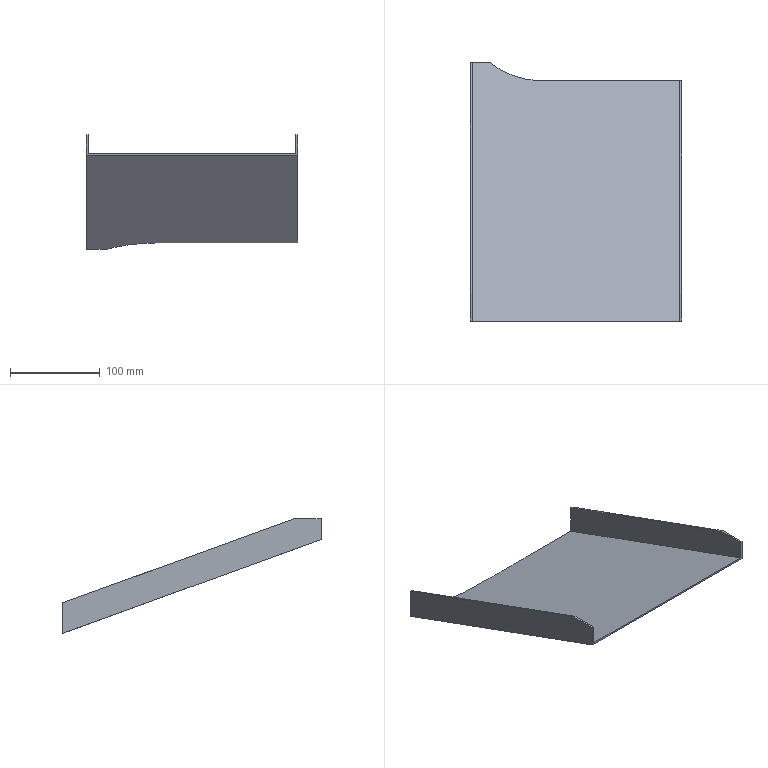Part | NX | features HB 2 | 1 solid | 14 faces | box 235 x 287.381 x 127.795 mm | volume 170241 mm3 | plane 13 | cylinder 1 | commonest cylinder face diameters 190 x1
STEP:
#1=CARTESIAN_POINT('',(799.54,-412.381,-213.));
#2=VERTEX_POINT('',#1);
#3=CARTESIAN_POINT('',(799.54,-382.551,-213.));
#4=VERTEX_POINT('',#3);
#5=CARTESIAN_POINT('',(799.54,-20.77,-213.));
#6=DIRECTION('',(0.,1.,0.));
#7=VECTOR('',#6,1000.);
#8=LINE('',#5,#7);
#9=EDGE_CURVE('',#2,#4,#8,.T.);
#10=ORIENTED_EDGE('',*,*,#9,.F.);
#11=CARTESIAN_POINT('',(799.54,-412.381,-236.196));
#12=VERTEX_POINT('',#11);
#13=CARTESIAN_POINT('',(799.54,-412.381,-376.603));
#14=DIRECTION('',(0.,0.,1.));
#15=VECTOR('',#14,1000.);
#16=LINE('',#13,#15);
#17=EDGE_CURVE('',#12,#2,#16,.T.);
#18=ORIENTED_EDGE('',*,*,#17,.F.);
#19=CARTESIAN_POINT('',(799.54,-145.,-333.515));
#20=VERTEX_POINT('',#19);
#21=CARTESIAN_POINT('',(799.54,-21.454,-378.482));
#22=DIRECTION('',(0.,0.9397,-0.342));
#23=VECTOR('',#22,1000.);
#24=LINE('',#21,#23);
#25=EDGE_CURVE('',#12,#20,#24,.T.);
#26=ORIENTED_EDGE('',*,*,#25,.T.);
#27=CARTESIAN_POINT('',(799.54,-145.,-299.462));
#28=VERTEX_POINT('',#27);
#29=CARTESIAN_POINT('',(799.54,-145.,-376.603));
#30=DIRECTION('',(0.,0.,1.));
#31=VECTOR('',#30,1000.);
#32=LINE('',#29,#31);
#33=EDGE_CURVE('',#20,#28,#32,.T.);
#34=ORIENTED_EDGE('',*,*,#33,.T.);
#35=CARTESIAN_POINT('',(799.54,-10.51,-348.412));
#36=DIRECTION('',(0.,-0.9397,0.342));
#37=VECTOR('',#36,1000.);
#38=LINE('',#35,#37);
#39=EDGE_CURVE('',#28,#4,#38,.T.);
#40=ORIENTED_EDGE('',*,*,#39,.T.);
#41=EDGE_LOOP('',(#10,#18,#26,#34,#40));
#42=FACE_BOUND('',#41,.T.);
#43=CARTESIAN_POINT('',(799.54,-20.77,-376.603));
#44=DIRECTION('',(-1.,0.,0.));
#45=DIRECTION('',(0.,0.08716,-0.9962));
#46=AXIS2_PLACEMENT_3D('',#43,#44,#45);
#47=PLANE('',#46);
#48=ADVANCED_FACE('',(#42),#47,.F.);
#49=CARTESIAN_POINT('',(797.54,-412.381,-234.068));
#50=VERTEX_POINT('',#49);
#51=CARTESIAN_POINT('',(797.54,-412.381,-213.));
#52=VERTEX_POINT('',#51);
#53=CARTESIAN_POINT('',(797.54,-412.381,-376.603));
#54=DIRECTION('',(0.,0.,1.));
#55=VECTOR('',#54,1000.);
#56=LINE('',#53,#55);
#57=EDGE_CURVE('',#50,#52,#56,.T.);
#58=ORIENTED_EDGE('',*,*,#57,.T.);
#59=CARTESIAN_POINT('',(797.54,-382.551,-213.));
#60=VERTEX_POINT('',#59);
#61=CARTESIAN_POINT('',(797.54,-20.77,-213.));
#62=DIRECTION('',(0.,1.,0.));
#63=VECTOR('',#62,1000.);
#64=LINE('',#61,#63);
#65=EDGE_CURVE('',#52,#60,#64,.T.);
#66=ORIENTED_EDGE('',*,*,#65,.T.);
#67=CARTESIAN_POINT('',(797.54,-145.,-299.462));
#68=VERTEX_POINT('',#67);
#69=CARTESIAN_POINT('',(797.54,-10.51,-348.412));
#70=DIRECTION('',(0.,-0.9397,0.342));
#71=VECTOR('',#70,1000.);
#72=LINE('',#69,#71);
#73=EDGE_CURVE('',#68,#60,#72,.T.);
#74=ORIENTED_EDGE('',*,*,#73,.F.);
#75=CARTESIAN_POINT('',(797.54,-145.,-331.387));
#76=VERTEX_POINT('',#75);
#77=CARTESIAN_POINT('',(797.54,-145.,-376.603));
#78=DIRECTION('',(0.,0.,1.));
#79=VECTOR('',#78,1000.);
#80=LINE('',#77,#79);
#81=EDGE_CURVE('',#76,#68,#80,.T.);
#82=ORIENTED_EDGE('',*,*,#81,.F.);
#83=CARTESIAN_POINT('',(797.54,-20.77,-376.603));
#84=DIRECTION('',(0.,-0.9397,0.342));
#85=VECTOR('',#84,1000.);
#86=LINE('',#83,#85);
#87=EDGE_CURVE('',#76,#50,#86,.T.);
#88=ORIENTED_EDGE('',*,*,#87,.T.);
#89=EDGE_LOOP('',(#58,#66,#74,#82,#88));
#90=FACE_BOUND('',#89,.T.);
#91=CARTESIAN_POINT('',(797.54,-20.77,-376.603));
#92=DIRECTION('',(-1.,0.,0.));
#93=DIRECTION('',(0.,-0.08716,0.9962));
#94=AXIS2_PLACEMENT_3D('',#91,#92,#93);
#95=PLANE('',#94);
#96=ADVANCED_FACE('',(#90),#95,.T.);
#97=CARTESIAN_POINT('',(907.54,-382.551,-213.));
#98=DIRECTION('',(-1.,0.,0.));
#99=VECTOR('',#98,1000.);
#100=LINE('',#97,#99);
#101=EDGE_CURVE('',#4,#60,#100,.T.);
#102=ORIENTED_EDGE('',*,*,#101,.F.);
#103=ORIENTED_EDGE('',*,*,#39,.F.);
#104=CARTESIAN_POINT('',(907.54,-145.,-299.462));
#105=DIRECTION('',(1.,0.,0.));
#106=VECTOR('',#105,1000.);
#107=LINE('',#104,#106);
#108=EDGE_CURVE('',#68,#28,#107,.T.);
#109=ORIENTED_EDGE('',*,*,#108,.F.);
#110=ORIENTED_EDGE('',*,*,#73,.T.);
#111=EDGE_LOOP('',(#102,#103,#109,#110));
#112=FACE_BOUND('',#111,.T.);
#113=CARTESIAN_POINT('',(907.54,-10.51,-348.412));
#114=DIRECTION('',(0.,-0.342,-0.9397));
#115=DIRECTION('',(0.,0.9397,-0.342));
#116=AXIS2_PLACEMENT_3D('',#113,#114,#115);
#117=PLANE('',#116);
#118=ADVANCED_FACE('',(#112),#117,.F.);
#119=CARTESIAN_POINT('',(564.54,-382.551,-213.));
#120=VERTEX_POINT('',#119);
#121=CARTESIAN_POINT('',(564.54,-412.381,-213.));
#122=VERTEX_POINT('',#121);
#123=CARTESIAN_POINT('',(564.54,-20.77,-213.));
#124=DIRECTION('',(0.,-1.,0.));
#125=VECTOR('',#124,1000.);
#126=LINE('',#123,#125);
#127=EDGE_CURVE('',#120,#122,#126,.T.);
#128=ORIENTED_EDGE('',*,*,#127,.F.);
#129=CARTESIAN_POINT('',(564.54,-125.,-306.741));
#130=VERTEX_POINT('',#129);
#131=CARTESIAN_POINT('',(564.54,-10.51,-348.412));
#132=DIRECTION('',(0.,-0.9397,0.342));
#133=VECTOR('',#132,1000.);
#134=LINE('',#131,#133);
#135=EDGE_CURVE('',#130,#120,#134,.T.);
#136=ORIENTED_EDGE('',*,*,#135,.F.);
#137=CARTESIAN_POINT('',(564.54,-125.,-340.795));
#138=VERTEX_POINT('',#137);
#139=CARTESIAN_POINT('',(564.54,-125.,-376.603));
#140=DIRECTION('',(0.,0.,-1.));
#141=VECTOR('',#140,1000.);
#142=LINE('',#139,#141);
#143=EDGE_CURVE('',#130,#138,#142,.T.);
#144=ORIENTED_EDGE('',*,*,#143,.T.);
#145=CARTESIAN_POINT('',(564.54,-412.381,-236.196));
#146=VERTEX_POINT('',#145);
#147=CARTESIAN_POINT('',(564.54,-21.454,-378.482));
#148=DIRECTION('',(0.,-0.9397,0.342));
#149=VECTOR('',#148,1000.);
#150=LINE('',#147,#149);
#151=EDGE_CURVE('',#138,#146,#150,.T.);
#152=ORIENTED_EDGE('',*,*,#151,.T.);
#153=CARTESIAN_POINT('',(564.54,-412.381,-376.603));
#154=DIRECTION('',(0.,0.,-1.));
#155=VECTOR('',#154,1000.);
#156=LINE('',#153,#155);
#157=EDGE_CURVE('',#122,#146,#156,.T.);
#158=ORIENTED_EDGE('',*,*,#157,.F.);
#159=EDGE_LOOP('',(#128,#136,#144,#152,#158));
#160=FACE_BOUND('',#159,.T.);
#161=CARTESIAN_POINT('',(564.54,-20.77,-376.603));
#162=DIRECTION('',(1.,0.,0.));
#163=DIRECTION('',(0.,-0.08716,0.9962));
#164=AXIS2_PLACEMENT_3D('',#161,#162,#163);
#165=PLANE('',#164);
#166=ADVANCED_FACE('',(#160),#165,.F.);
#167=CARTESIAN_POINT('',(566.54,-125.,-306.741));
#168=VERTEX_POINT('',#167);
#169=CARTESIAN_POINT('',(566.54,-382.551,-213.));
#170=VERTEX_POINT('',#169);
#171=CARTESIAN_POINT('',(566.54,-10.51,-348.412));
#172=DIRECTION('',(0.,-0.9397,0.342));
#173=VECTOR('',#172,1000.);
#174=LINE('',#171,#173);
#175=EDGE_CURVE('',#168,#170,#174,.T.);
#176=ORIENTED_EDGE('',*,*,#175,.T.);
#177=CARTESIAN_POINT('',(566.54,-412.381,-213.));
#178=VERTEX_POINT('',#177);
#179=CARTESIAN_POINT('',(566.54,-20.77,-213.));
#180=DIRECTION('',(0.,-1.,0.));
#181=VECTOR('',#180,1000.);
#182=LINE('',#179,#181);
#183=EDGE_CURVE('',#170,#178,#182,.T.);
#184=ORIENTED_EDGE('',*,*,#183,.T.);
#185=CARTESIAN_POINT('',(566.54,-412.381,-234.068));
#186=VERTEX_POINT('',#185);
#187=CARTESIAN_POINT('',(566.54,-412.381,-376.603));
#188=DIRECTION('',(0.,0.,-1.));
#189=VECTOR('',#188,1000.);
#190=LINE('',#187,#189);
#191=EDGE_CURVE('',#178,#186,#190,.T.);
#192=ORIENTED_EDGE('',*,*,#191,.T.);
#193=CARTESIAN_POINT('',(566.54,-125.,-338.666));
#194=VERTEX_POINT('',#193);
#195=CARTESIAN_POINT('',(566.54,-20.77,-376.603));
#196=DIRECTION('',(0.,0.9397,-0.342));
#197=VECTOR('',#196,1000.);
#198=LINE('',#195,#197);
#199=EDGE_CURVE('',#186,#194,#198,.T.);
#200=ORIENTED_EDGE('',*,*,#199,.T.);
#201=CARTESIAN_POINT('',(566.54,-125.,-376.603));
#202=DIRECTION('',(0.,0.,-1.));
#203=VECTOR('',#202,1000.);
#204=LINE('',#201,#203);
#205=EDGE_CURVE('',#168,#194,#204,.T.);
#206=ORIENTED_EDGE('',*,*,#205,.F.);
#207=EDGE_LOOP('',(#176,#184,#192,#200,#206));
#208=FACE_BOUND('',#207,.T.);
#209=CARTESIAN_POINT('',(566.54,-20.77,-376.603));
#210=DIRECTION('',(1.,0.,0.));
#211=DIRECTION('',(0.,-0.08716,0.9962));
#212=AXIS2_PLACEMENT_3D('',#209,#210,#211);
#213=PLANE('',#212);
#214=ADVANCED_FACE('',(#208),#213,.T.);
#215=CARTESIAN_POINT('',(564.54,-382.551,-213.));
#216=DIRECTION('',(-1.,0.,0.));
#217=VECTOR('',#216,1000.);
#218=LINE('',#215,#217);
#219=EDGE_CURVE('',#170,#120,#218,.T.);
#220=ORIENTED_EDGE('',*,*,#219,.F.);
#221=ORIENTED_EDGE('',*,*,#175,.F.);
#222=CARTESIAN_POINT('',(564.54,-125.,-306.741));
#223=DIRECTION('',(-1.,0.,0.));
#224=VECTOR('',#223,1000.);
#225=LINE('',#222,#224);
#226=EDGE_CURVE('',#168,#130,#225,.T.);
#227=ORIENTED_EDGE('',*,*,#226,.T.);
#228=ORIENTED_EDGE('',*,*,#135,.T.);
#229=EDGE_LOOP('',(#220,#221,#227,#228));
#230=FACE_BOUND('',#229,.T.);
#231=CARTESIAN_POINT('',(564.54,-10.51,-348.412));
#232=DIRECTION('',(0.,-0.342,-0.9397));
#233=DIRECTION('',(0.,0.9397,-0.342));
#234=AXIS2_PLACEMENT_3D('',#231,#232,#233);
#235=PLANE('',#234);
#236=ADVANCED_FACE('',(#230),#235,.F.);
#237=ORIENTED_EDGE('',*,*,#17,.T.);
#238=CARTESIAN_POINT('',(293.54,-412.381,-213.));
#239=DIRECTION('',(-1.,0.,0.));
#240=VECTOR('',#239,1000.);
#241=LINE('',#238,#240);
#242=EDGE_CURVE('',#2,#52,#241,.T.);
#243=ORIENTED_EDGE('',*,*,#242,.T.);
#244=ORIENTED_EDGE('',*,*,#57,.F.);
#245=CARTESIAN_POINT('',(796.54,-412.381,-234.068));
#246=DIRECTION('',(1.,0.,0.));
#247=VECTOR('',#246,1000.);
#248=LINE('',#245,#247);
#249=EDGE_CURVE('',#186,#50,#248,.T.);
#250=ORIENTED_EDGE('',*,*,#249,.F.);
#251=ORIENTED_EDGE('',*,*,#191,.F.);
#252=CARTESIAN_POINT('',(287.54,-412.381,-213.));
#253=DIRECTION('',(-1.,0.,0.));
#254=VECTOR('',#253,1000.);
#255=LINE('',#252,#254);
#256=EDGE_CURVE('',#178,#122,#255,.T.);
#257=ORIENTED_EDGE('',*,*,#256,.T.);
#258=ORIENTED_EDGE('',*,*,#157,.T.);
#259=CARTESIAN_POINT('',(796.54,-412.381,-236.196));
#260=DIRECTION('',(1.,0.,0.));
#261=VECTOR('',#260,1000.);
#262=LINE('',#259,#261);
#263=EDGE_CURVE('',#146,#12,#262,.T.);
#264=ORIENTED_EDGE('',*,*,#263,.T.);
#265=EDGE_LOOP('',(#237,#243,#244,#250,#251,#257,#258,#264));
#266=FACE_BOUND('',#265,.T.);
#267=CARTESIAN_POINT('',(287.54,-412.381,0.));
#268=DIRECTION('',(0.,-1.,0.));
#269=DIRECTION('',(0.,0.,-1.));
#270=AXIS2_PLACEMENT_3D('',#267,#268,#269);
#271=PLANE('',#270);
#272=ADVANCED_FACE('',(#266),#271,.T.);
#273=CARTESIAN_POINT('',(586.69,-125.,-338.666));
#274=VERTEX_POINT('',#273);
#275=CARTESIAN_POINT('',(796.54,-125.,-338.666));
#276=DIRECTION('',(1.,0.,0.));
#277=VECTOR('',#276,1000.);
#278=LINE('',#275,#277);
#279=EDGE_CURVE('',#194,#274,#278,.T.);
#280=ORIENTED_EDGE('',*,*,#279,.T.);
#281=CARTESIAN_POINT('',(586.69,-125.,-340.795));
#282=VERTEX_POINT('',#281);
#283=CARTESIAN_POINT('',(586.69,-125.,-1480.5));
#284=DIRECTION('',(0.,0.,1.));
#285=VECTOR('',#284,1000.);
#286=LINE('',#283,#285);
#287=EDGE_CURVE('',#282,#274,#286,.T.);
#288=ORIENTED_EDGE('',*,*,#287,.F.);
#289=CARTESIAN_POINT('',(796.54,-125.,-340.795));
#290=DIRECTION('',(1.,0.,0.));
#291=VECTOR('',#290,1000.);
#292=LINE('',#289,#291);
#293=EDGE_CURVE('',#138,#282,#292,.T.);
#294=ORIENTED_EDGE('',*,*,#293,.F.);
#295=ORIENTED_EDGE('',*,*,#143,.F.);
#296=ORIENTED_EDGE('',*,*,#226,.F.);
#297=ORIENTED_EDGE('',*,*,#205,.T.);
#298=EDGE_LOOP('',(#280,#288,#294,#295,#296,#297));
#299=FACE_BOUND('',#298,.T.);
#300=CARTESIAN_POINT('',(1033.,-125.,-2230.5));
#301=DIRECTION('',(0.,-1.,0.));
#302=DIRECTION('',(0.,0.,-1.));
#303=AXIS2_PLACEMENT_3D('',#300,#301,#302);
#304=PLANE('',#303);
#305=ADVANCED_FACE('',(#299),#304,.F.);
#306=ORIENTED_EDGE('',*,*,#87,.F.);
#307=CARTESIAN_POINT('',(645.,-145.,-331.387));
#308=VERTEX_POINT('',#307);
#309=CARTESIAN_POINT('',(796.54,-145.,-331.387));
#310=DIRECTION('',(-1.,0.,0.));
#311=VECTOR('',#310,1000.);
#312=LINE('',#309,#311);
#313=EDGE_CURVE('',#76,#308,#312,.T.);
#314=ORIENTED_EDGE('',*,*,#313,.T.);
#315=CARTESIAN_POINT('',(645.,-50.,-365.964));
#316=DIRECTION('',(0.,-0.342,-0.9397));
#317=DIRECTION('',(0.,-0.9397,0.342));
#318=AXIS2_PLACEMENT_3D('',#315,#316,#317);
#319=ELLIPSE('',#318,101.097,95.);
#320=EDGE_CURVE('',#308,#274,#319,.T.);
#321=ORIENTED_EDGE('',*,*,#320,.T.);
#322=ORIENTED_EDGE('',*,*,#279,.F.);
#323=ORIENTED_EDGE('',*,*,#199,.F.);
#324=ORIENTED_EDGE('',*,*,#249,.T.);
#325=EDGE_LOOP('',(#306,#314,#321,#322,#323,#324));
#326=FACE_BOUND('',#325,.T.);
#327=CARTESIAN_POINT('',(796.54,-20.77,-376.603));
#328=DIRECTION('',(0.,0.342,0.9397));
#329=DIRECTION('',(-1.,0.,0.));
#330=AXIS2_PLACEMENT_3D('',#327,#328,#329);
#331=PLANE('',#330);
#332=ADVANCED_FACE('',(#326),#331,.T.);
#333=CARTESIAN_POINT('',(645.,-145.,-333.515));
#334=VERTEX_POINT('',#333);
#335=CARTESIAN_POINT('',(796.54,-145.,-333.515));
#336=DIRECTION('',(1.,0.,0.));
#337=VECTOR('',#336,1000.);
#338=LINE('',#335,#337);
#339=EDGE_CURVE('',#334,#20,#338,.T.);
#340=ORIENTED_EDGE('',*,*,#339,.T.);
#341=ORIENTED_EDGE('',*,*,#25,.F.);
#342=ORIENTED_EDGE('',*,*,#263,.F.);
#343=ORIENTED_EDGE('',*,*,#151,.F.);
#344=ORIENTED_EDGE('',*,*,#293,.T.);
#345=CARTESIAN_POINT('',(645.,-50.,-368.092));
#346=DIRECTION('',(0.,-0.342,-0.9397));
#347=DIRECTION('',(0.,-0.9397,0.342));
#348=AXIS2_PLACEMENT_3D('',#345,#346,#347);
#349=ELLIPSE('',#348,101.097,95.);
#350=EDGE_CURVE('',#334,#282,#349,.T.);
#351=ORIENTED_EDGE('',*,*,#350,.F.);
#352=EDGE_LOOP('',(#340,#341,#342,#343,#344,#351));
#353=FACE_BOUND('',#352,.T.);
#354=CARTESIAN_POINT('',(796.54,-21.454,-378.482));
#355=DIRECTION('',(0.,0.342,0.9397));
#356=DIRECTION('',(-1.,0.,0.));
#357=AXIS2_PLACEMENT_3D('',#354,#355,#356);
#358=PLANE('',#357);
#359=ADVANCED_FACE('',(#353),#358,.F.);
#360=ORIENTED_EDGE('',*,*,#313,.F.);
#361=ORIENTED_EDGE('',*,*,#81,.T.);
#362=ORIENTED_EDGE('',*,*,#108,.T.);
#363=ORIENTED_EDGE('',*,*,#33,.F.);
#364=ORIENTED_EDGE('',*,*,#339,.F.);
#365=CARTESIAN_POINT('',(645.,-145.,-1480.5));
#366=DIRECTION('',(0.,0.,1.));
#367=VECTOR('',#366,1000.);
#368=LINE('',#365,#367);
#369=EDGE_CURVE('',#334,#308,#368,.T.);
#370=ORIENTED_EDGE('',*,*,#369,.T.);
#371=EDGE_LOOP('',(#360,#361,#362,#363,#364,#370));
#372=FACE_BOUND('',#371,.T.);
#373=CARTESIAN_POINT('',(845.,-145.,-1480.5));
#374=DIRECTION('',(0.,1.,0.));
#375=DIRECTION('',(0.,0.,-1.));
#376=AXIS2_PLACEMENT_3D('',#373,#374,#375);
#377=PLANE('',#376);
#378=ADVANCED_FACE('',(#372),#377,.T.);
#379=ORIENTED_EDGE('',*,*,#320,.F.);
#380=ORIENTED_EDGE('',*,*,#369,.F.);
#381=ORIENTED_EDGE('',*,*,#350,.T.);
#382=ORIENTED_EDGE('',*,*,#287,.T.);
#383=EDGE_LOOP('',(#379,#380,#381,#382));
#384=FACE_BOUND('',#383,.T.);
#385=CARTESIAN_POINT('',(645.,-50.,-1480.5));
#386=DIRECTION('',(0.,0.,1.));
#387=DIRECTION('',(-1.,0.,0.));
#388=AXIS2_PLACEMENT_3D('',#385,#386,#387);
#389=CYLINDRICAL_SURFACE('',#388,95.);
#390=ADVANCED_FACE('',(#384),#389,.F.);
#391=ORIENTED_EDGE('',*,*,#183,.F.);
#392=ORIENTED_EDGE('',*,*,#219,.T.);
#393=ORIENTED_EDGE('',*,*,#127,.T.);
#394=ORIENTED_EDGE('',*,*,#256,.F.);
#395=EDGE_LOOP('',(#391,#392,#393,#394));
#396=FACE_BOUND('',#395,.T.);
#397=CARTESIAN_POINT('',(1945.,0.,-213.));
#398=DIRECTION('',(0.,0.,1.));
#399=DIRECTION('',(-1.,0.,0.));
#400=AXIS2_PLACEMENT_3D('',#397,#398,#399);
#401=PLANE('',#400);
#402=ADVANCED_FACE('',(#396),#401,.T.);
#403=ORIENTED_EDGE('',*,*,#9,.T.);
#404=ORIENTED_EDGE('',*,*,#101,.T.);
#405=ORIENTED_EDGE('',*,*,#65,.F.);
#406=ORIENTED_EDGE('',*,*,#242,.F.);
#407=EDGE_LOOP('',(#403,#404,#405,#406));
#408=FACE_BOUND('',#407,.T.);
#409=CARTESIAN_POINT('',(1951.,0.,-213.));
#410=DIRECTION('',(0.,0.,1.));
#411=DIRECTION('',(-1.,0.,0.));
#412=AXIS2_PLACEMENT_3D('',#409,#410,#411);
#413=PLANE('',#412);
#414=ADVANCED_FACE('',(#408),#413,.T.);
#415=CLOSED_SHELL('',(#48,#96,#118,#166,#214,#236,#272,#305,#332,#359,#378,#390,#402,#414));
#416=MANIFOLD_SOLID_BREP('',#415);
#417=(LENGTH_UNIT()NAMED_UNIT(*)SI_UNIT(.MILLI.,.METRE.));
#418=UNCERTAINTY_MEASURE_WITH_UNIT(LENGTH_MEASURE(0.00001),#417,'','');
#419=(NAMED_UNIT(*)PLANE_ANGLE_UNIT()SI_UNIT($,.RADIAN.));
#420=(NAMED_UNIT(*)SI_UNIT($,.STERADIAN.)SOLID_ANGLE_UNIT());
#421=(GEOMETRIC_REPRESENTATION_CONTEXT(3)GLOBAL_UNCERTAINTY_ASSIGNED_CONTEXT((#418))GLOBAL_UNIT_ASSIGNED_CONTEXT((#417,#419,#420))REPRESENTATION_CONTEXT('',''));
#422=ADVANCED_BREP_SHAPE_REPRESENTATION('',(#416),#421);